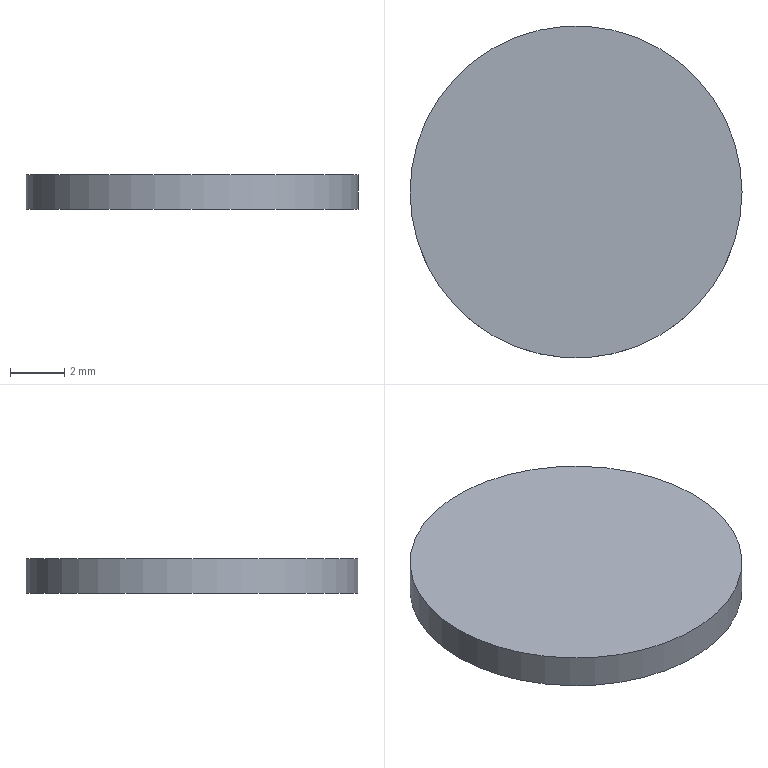Part | STEP file | gslz 2016.10.28-13_id1178_x_t | 1 solid | 3 faces | box 12.2 x 12.2 x 1.25 mm | volume 146.123 mm3 | plane 2 | cylinder 1 | commonest cylinder face diameters 12.2 x1
STEP:
#1=CARTESIAN_POINT('',(0.,0.,0.));
#2=DIRECTION('',(0.,0.,1.));
#3=DIRECTION('',(1.,0.,0.));
#4=AXIS2_PLACEMENT_3D('',#1,#2,#3);
#5=CARTESIAN_POINT('',(-1417.272,254.,1.25));
#6=VERTEX_POINT('',#5);
#7=CARTESIAN_POINT('',(-1423.372,254.,1.25));
#8=DIRECTION('',(0.,0.,1.));
#9=DIRECTION('',(1.,0.,0.));
#10=AXIS2_PLACEMENT_3D('',#7,#8,#9);
#11=CIRCLE('',#10,6.1);
#12=CARTESIAN_POINT('',(-1423.372,254.,3.25));
#13=DIRECTION('',(0.,0.,-1.));
#14=DIRECTION('',(-1.,0.,0.));
#15=AXIS2_PLACEMENT_3D('',#12,#13,#14);
#16=CYLINDRICAL_SURFACE('',#15,6.1);
#17=CARTESIAN_POINT('',(9.425,2.));
#18=DIRECTION('',(-1.,0.));
#19=VECTOR('',#18,1.);
#20=LINE('',#17,#19);
#21=(GEOMETRIC_REPRESENTATION_CONTEXT(2)PARAMETRIC_REPRESENTATION_CONTEXT()REPRESENTATION_CONTEXT('',''));
#22=DEFINITIONAL_REPRESENTATION('',(#20),#21);
#23=PCURVE('',#16,#22);
#24=CARTESIAN_POINT('',(-1423.372,254.,1.25));
#25=DIRECTION('',(0.,0.,1.));
#26=DIRECTION('',(1.,0.,0.));
#27=AXIS2_PLACEMENT_3D('',#24,#25,#26);
#28=PLANE('',#27);
#29=CARTESIAN_POINT('',(0.,0.));
#30=DIRECTION('',(1.,0.));
#31=AXIS2_PLACEMENT_2D('',#29,#30);
#32=CIRCLE('',#31,6.1);
#33=(GEOMETRIC_REPRESENTATION_CONTEXT(2)PARAMETRIC_REPRESENTATION_CONTEXT()REPRESENTATION_CONTEXT('',''));
#34=DEFINITIONAL_REPRESENTATION('',(#32),#33);
#35=PCURVE('',#28,#34);
#36=SURFACE_CURVE('',#11,(#23,#35),.PCURVE_S1.);
#37=EDGE_CURVE('',#6,#6,#36,.T.);
#38=ORIENTED_EDGE('',*,*,#37,.F.);
#39=CARTESIAN_POINT('',(-1417.272,254.,0.));
#40=VERTEX_POINT('',#39);
#41=CARTESIAN_POINT('',(-1417.272,254.,1.25));
#42=CARTESIAN_POINT('',(-1417.272,254.,0.));
#43=B_SPLINE_CURVE_WITH_KNOTS('',1,(#41,#42),.UNSPECIFIED.,.F.,.F.,(2,2),(2.,3.25),.PIECEWISE_BEZIER_KNOTS.);
#44=CARTESIAN_POINT('',(9.425,0.));
#45=DIRECTION('',(0.,1.));
#46=VECTOR('',#45,1.);
#47=LINE('',#44,#46);
#48=(GEOMETRIC_REPRESENTATION_CONTEXT(2)PARAMETRIC_REPRESENTATION_CONTEXT()REPRESENTATION_CONTEXT('',''));
#49=DEFINITIONAL_REPRESENTATION('',(#47),#48);
#50=PCURVE('',#16,#49);
#51=CARTESIAN_POINT('',(3.142,0.));
#52=DIRECTION('',(0.,1.));
#53=VECTOR('',#52,1.);
#54=LINE('',#51,#53);
#55=(GEOMETRIC_REPRESENTATION_CONTEXT(2)PARAMETRIC_REPRESENTATION_CONTEXT()REPRESENTATION_CONTEXT('',''));
#56=DEFINITIONAL_REPRESENTATION('',(#54),#55);
#57=PCURVE('',#16,#56);
#58=SEAM_CURVE('',#43,(#50,#57),.PCURVE_S1.);
#59=EDGE_CURVE('',#6,#40,#58,.T.);
#60=ORIENTED_EDGE('',*,*,#59,.T.);
#61=CARTESIAN_POINT('',(-1423.372,254.,0.));
#62=DIRECTION('',(0.,0.,1.));
#63=DIRECTION('',(1.,0.,0.));
#64=AXIS2_PLACEMENT_3D('',#61,#62,#63);
#65=CIRCLE('',#64,6.1);
#66=CARTESIAN_POINT('',(9.425,3.25));
#67=DIRECTION('',(-1.,0.));
#68=VECTOR('',#67,1.);
#69=LINE('',#66,#68);
#70=(GEOMETRIC_REPRESENTATION_CONTEXT(2)PARAMETRIC_REPRESENTATION_CONTEXT()REPRESENTATION_CONTEXT('',''));
#71=DEFINITIONAL_REPRESENTATION('',(#69),#70);
#72=PCURVE('',#16,#71);
#73=CARTESIAN_POINT('',(-1423.372,254.,0.));
#74=DIRECTION('',(0.,0.,1.));
#75=DIRECTION('',(1.,0.,0.));
#76=AXIS2_PLACEMENT_3D('',#73,#74,#75);
#77=PLANE('',#76);
#78=CARTESIAN_POINT('',(0.,0.));
#79=DIRECTION('',(1.,0.));
#80=AXIS2_PLACEMENT_2D('',#78,#79);
#81=CIRCLE('',#80,6.1);
#82=(GEOMETRIC_REPRESENTATION_CONTEXT(2)PARAMETRIC_REPRESENTATION_CONTEXT()REPRESENTATION_CONTEXT('',''));
#83=DEFINITIONAL_REPRESENTATION('',(#81),#82);
#84=PCURVE('',#77,#83);
#85=SURFACE_CURVE('',#65,(#72,#84),.PCURVE_S1.);
#86=EDGE_CURVE('',#40,#40,#85,.T.);
#87=ORIENTED_EDGE('',*,*,#86,.T.);
#88=ORIENTED_EDGE('',*,*,#59,.F.);
#89=EDGE_LOOP('',(#38,#60,#87,#88));
#90=FACE_BOUND('',#89,.T.);
#91=ADVANCED_FACE('',(#90),#16,.T.);
#92=ORIENTED_EDGE('',*,*,#37,.T.);
#93=EDGE_LOOP('',(#92));
#94=FACE_BOUND('',#93,.T.);
#95=ADVANCED_FACE('',(#94),#28,.T.);
#96=ORIENTED_EDGE('',*,*,#86,.F.);
#97=EDGE_LOOP('',(#96));
#98=FACE_BOUND('',#97,.T.);
#99=ADVANCED_FACE('',(#98),#77,.F.);
#100=CLOSED_SHELL('',(#91,#95,#99));
#101=MANIFOLD_SOLID_BREP('',#100);
#102=(LENGTH_UNIT()NAMED_UNIT(*)SI_UNIT(.MILLI.,.METRE.));
#103=UNCERTAINTY_MEASURE_WITH_UNIT(LENGTH_MEASURE(0.00001),#102,'','');
#104=(NAMED_UNIT(*)PLANE_ANGLE_UNIT()SI_UNIT($,.RADIAN.));
#105=(NAMED_UNIT(*)SI_UNIT($,.STERADIAN.)SOLID_ANGLE_UNIT());
#106=(GEOMETRIC_REPRESENTATION_CONTEXT(3)GLOBAL_UNCERTAINTY_ASSIGNED_CONTEXT((#103))GLOBAL_UNIT_ASSIGNED_CONTEXT((#102,#104,#105))REPRESENTATION_CONTEXT('',''));
#107=ADVANCED_BREP_SHAPE_REPRESENTATION('',(#4,#101),#106);